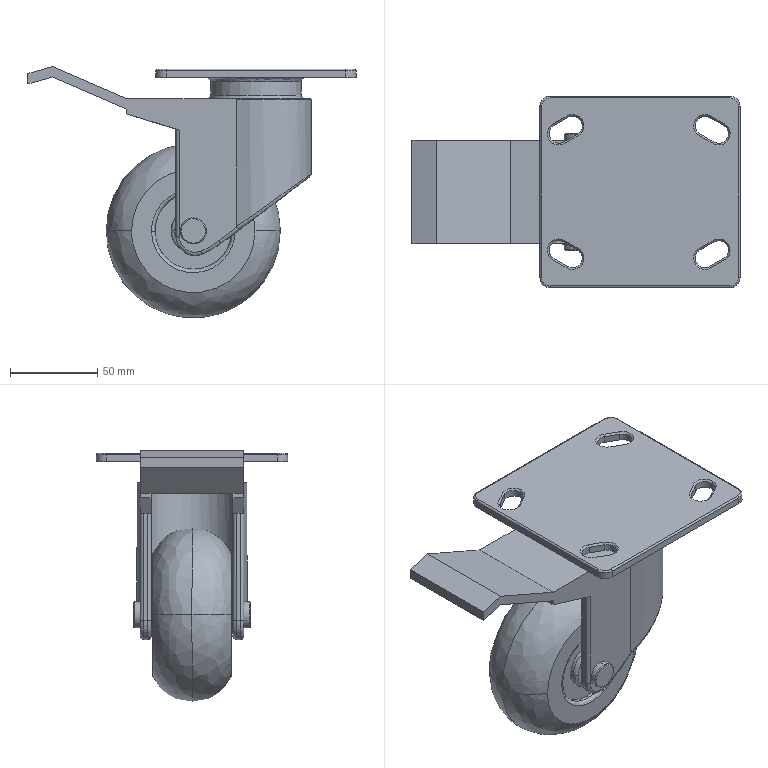Part | STEP file | QA-KVJHX100-1 | 1 solid | 155 faces | box 188.5 x 110 x 144.462 mm | volume 504709 mm3 | cylinder 54 | plane 52 | spline 33 | cone 16 | commonest cylinder face diameters 11 x12 4 x8 15 x8 2 x4 12 x4 22 x4